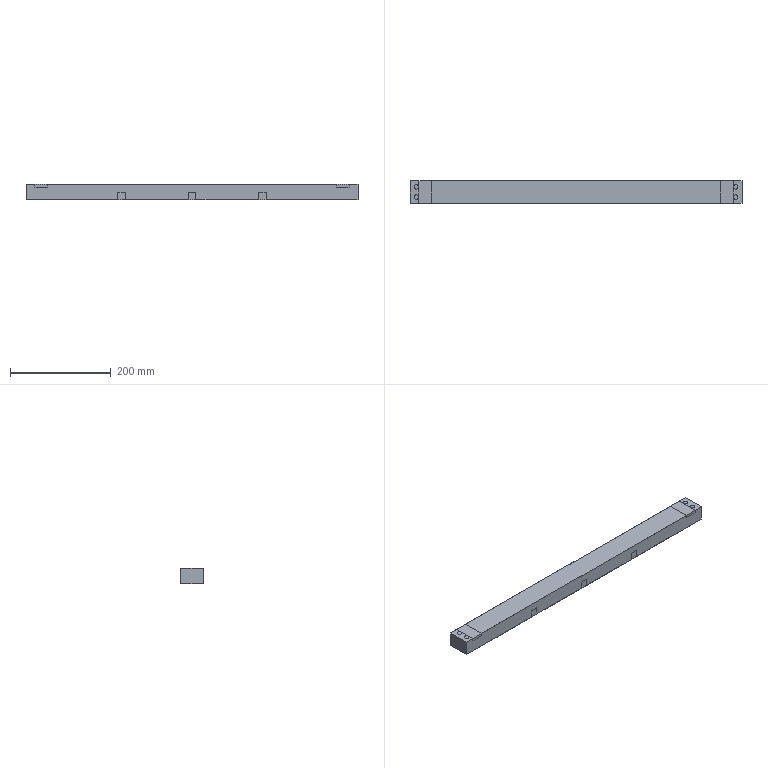NC program | NX | posted with a generic post | part box 659.9 x 45 x 30 mm
Whole program:
N10 G17 G21 G94 G90
(FLOOR_WALL , TOOL : D63)
N12 T01 M6
N14 G54
N16 G17 G0 G90 X-366.45 Y0. S6500 M3
N18 G43 Z30. H1
N20 Z3.
N22 G94 G1 Z0. F1250.
N24 X-363.45
N26 X363.45
N28 X366.45
N30 Z3.
N32 G0 Z30.
N34 M5
(ZLEVEL_PROFILE_COPY_2 , TOOL : D12)
N36 T20 M6
N38 G54
N40 G17 G0 G90 X338.221 Y33.444 S8000 M3
N42 G43 Z30. H20
N44 Z-1.
N46 G94 G1 X336.646 Y32.535 F3500.
N48 G3 X336.046 Y31.496 R1.2
N50 G1 Y23.409
N52 X336.05 Y22.53
N54 Y-17.291
N56 X336.046 Y-17.344
N58 Y-31.496
N60 G3 X336.646 Y-32.535 R1.2
N62 G1 X338.221 Y-33.444
N64 G0 Z-2.
N66 G1 X336.646 Y-32.535
N68 G2 X336.046 Y-31.496 R1.2
N70 G1 Y-17.344
N72 X336.05 Y-17.291
N74 Y22.53
N76 X336.046 Y23.409
N78 Y31.496
N80 G2 X336.646 Y32.535 R1.2
N82 G1 X338.221 Y33.444
N84 G0 Z-3.
N86 G1 X336.646 Y32.535
N88 G3 X336.046 Y31.496 R1.2
N90 G1 Y23.409
N92 X336.05 Y22.53
N94 Y-17.291
N96 X336.046 Y-17.344
N98 Y-31.496
N100 G3 X336.646 Y-32.535 R1.2
N102 G1 X338.221 Y-33.444
N104 G0 Z-4.
N106 G1 X336.646 Y-32.535
N108 G2 X336.046 Y-31.496 R1.2
N110 G1 Y-17.344
N112 X336.05 Y-17.291
N114 Y22.53
N116 X336.046 Y23.409
N118 Y31.496
N120 G2 X336.646 Y32.535 R1.2
N122 G1 X338.221 Y33.444
N124 G0 Z-5.
N126 G1 X336.646 Y32.535
N128 G3 X336.046 Y31.496 R1.2
N130 G1 Y23.409
N132 X336.05 Y22.53
N134 Y-17.291
N136 X336.046 Y-17.344
N138 Y-31.496
N140 G3 X336.646 Y-32.535 R1.2
N142 G1 X338.221 Y-33.444
N144 G0 Z-6.
N146 G1 X336.646 Y-32.535
N148 G2 X336.046 Y-31.496 R1.2
N150 G1 Y-17.344
N152 X336.05 Y-17.291
N154 Y22.53
N156 X336.046 Y23.409
N158 Y31.496
N160 G2 X336.646 Y32.535 R1.2
N162 G1 X338.221 Y33.444
N164 G0 Z-7.
N166 G1 X336.646 Y32.535
N168 G3 X336.046 Y31.496 R1.2
N170 G1 Y23.409
N172 X336.05 Y22.53
N174 Y-17.291
N176 X336.046 Y-17.344
N178 Y-31.496
N180 G3 X336.646 Y-32.535 R1.2
N182 G1 X338.221 Y-33.444
N184 G0 Z-8.
N186 G1 X336.647 Y-32.535
N188 G2 X336.047 Y-31.496 R1.2
N190 G1 Y-17.344
N192 X336.05 Y-17.291
N194 Y22.53
N196 X336.047 Y23.409
N198 Y31.496
N200 G2 X336.647 Y32.535 R1.2
N202 G1 X338.221 Y33.444
N204 G0 Z-9.
N206 G1 X336.647 Y32.535
N208 G3 X336.047 Y31.496 R1.2
N210 G1 Y23.409
N212 X336.05 Y22.53
N214 Y-17.291
N216 X336.047 Y-17.344
N218 Y-31.496
N220 G3 X336.647 Y-32.535 R1.2
N222 G1 X338.221 Y-33.444
N224 G0 Z-10.
N226 G1 X336.647 Y-32.535
N228 G2 X336.047 Y-31.496 R1.2
N230 G1 Y-17.344
N232 X336.05 Y-17.291
N234 Y22.53
N236 X336.047 Y23.409
N238 Y31.496
N240 G2 X336.647 Y32.535 R1.2
N242 G1 X338.221 Y33.444
N244 G0 Z-11.
N246 G1 X336.647 Y32.535
N248 G3 X336.047 Y31.496 R1.2
N250 G1 Y23.409
N252 X336.05 Y22.53
N254 Y-17.291
N256 X336.047 Y-17.344
N258 Y-31.496
N260 G3 X336.647 Y-32.535 R1.2
N262 G1 X338.221 Y-33.444
N264 G0 Z-12.
N266 G1 X336.647 Y-32.535
N268 G2 X336.047 Y-31.496 R1.2
N270 G1 Y-17.344
N272 X336.05 Y-17.291
N274 Y22.53
N276 X336.047 Y23.409
N278 Y31.496
N280 G2 X336.647 Y32.535 R1.2
N282 G1 X338.222 Y33.444
N284 G0 Z-13.
N286 G1 X336.647 Y32.535
N288 G3 X336.047 Y31.496 R1.2
N290 G1 Y23.409
N292 X336.05 Y22.53
N294 X336.047 Y-17.344
N296 Y-31.496
N298 G3 X336.647 Y-32.535 R1.2
N300 G1 X338.222 Y-33.444
N302 G0 Z-14.
N304 G1 X336.647 Y-32.535
N306 G2 X336.047 Y-31.496 R1.2
N308 G1 X336.05 Y-17.291
N310 Y22.53
N312 X336.047 Y23.409
N314 Y31.496
N316 G2 X336.647 Y32.535 R1.2
N318 G1 X338.222 Y33.444
N320 G0 Z-15.
N322 G1 X336.647 Y32.535
N324 G3 X336.047 Y31.496 R1.2
N326 G1 Y23.409
N328 X336.05 Y22.53
N330 X336.047 Y-17.344
N332 Y-31.496
N334 G3 X336.647 Y-32.535 R1.2
N336 G1 X338.222 Y-33.444
N338 G0 Z-16.
N340 G1 X336.647 Y-32.535
N342 G2 X336.047 Y-31.496 R1.2
N344 G1 X336.05 Y-17.291
N346 Y22.53
N348 X336.047 Y23.409
N350 Y31.496
N352 G2 X336.647 Y32.535 R1.2
N354 G1 X338.222 Y33.444
N356 G0 Z-17.
N358 G1 X336.647 Y32.535
N360 G3 X336.047 Y31.496 R1.2
N362 G1 Y23.409
N364 X336.05 Y22.53
N366 X336.047 Y-17.344
N368 Y-31.496
N370 G3 X336.647 Y-32.535 R1.2
N372 G1 X338.222 Y-33.444
N374 G0 Z-18.
N376 G1 X336.647 Y-32.535
N378 G2 X336.047 Y-31.496 R1.2
N380 G1 X336.05 Y-17.291
N382 Y22.53
N384 X336.047 Y23.409
N386 Y31.496
N388 G2 X336.647 Y32.535 R1.2
N390 G1 X338.222 Y33.444
N392 G0 Z-19.
N394 G1 X336.648 Y32.535
N396 G3 X336.048 Y31.496 R1.2
N398 G1 Y23.409
N400 X336.05 Y22.53
N402 X336.048 Y-17.344
N404 Y-31.496
N406 G3 X336.648 Y-32.535 R1.2
N408 G1 X338.222 Y-33.444
N410 G0 Z-20.
N412 G1 X336.648 Y-32.535
N414 G2 X336.048 Y-31.496 R1.2
N416 G1 X336.05 Y-17.291
N418 Y22.53
N420 X336.048 Y23.409
N422 Y31.496
N424 G2 X336.648 Y32.535 R1.2
N426 G1 X338.222 Y33.444
N428 G0 Z-21.
N430 G1 X336.648 Y32.535
N432 G3 X336.048 Y31.496 R1.2
N434 G1 Y23.409
N436 X336.05 Y22.53
N438 X336.048 Y-17.344
N440 Y-31.496
N442 G3 X336.648 Y-32.535 R1.2
N444 G1 X338.222 Y-33.444
N446 G0 Z-22.
N448 G1 X336.648 Y-32.535
N450 G2 X336.048 Y-31.496 R1.2
N452 G1 X336.05 Y-17.291
N454 Y22.53
N456 X336.048 Y23.409
N458 Y31.496
N460 G2 X336.648 Y32.535 R1.2
N462 G1 X338.222 Y33.444
N464 G0 Y33.445 Z-23.
N466 G1 X336.648 Y32.536
N468 G3 X336.048 Y31.496 R1.2
N470 G1 X336.05 Y22.53
N472 X336.048 Y-17.344
N474 Y-31.496
N476 G3 X336.648 Y-32.535 R1.2
N478 G1 X338.222 Y-33.444
N480 G0 Z-24.
N482 G1 X336.648 Y-32.535
N484 G2 X336.048 Y-31.496 R1.2
N486 G1 X336.05 Y-17.291
N488 Y22.53
N490 X336.048 Y31.496
N492 G2 X336.648 Y32.536 R1.2
N494 G1 X338.222 Y33.445
N496 G0 Z-25.
N498 G1 X336.648 Y32.536
N500 G3 X336.048 Y31.496 R1.2
N502 G1 X336.05 Y22.53
N504 X336.048 Y-17.344
N506 Y-31.496
N508 G3 X336.648 Y-32.535 R1.2
N510 G1 X338.222 Y-33.444
N512 G0 X338.223 Y-33.445 Z-26.
N514 G1 X336.648 Y-32.535
N516 G2 X336.048 Y-31.496 R1.2
N518 G1 X336.05 Y-17.291
N520 Y22.53
N522 X336.048 Y31.496
N524 G2 X336.648 Y32.536 R1.2
N526 G1 X338.223 Y33.445
N528 G0 Z-27.
N530 G1 X336.648 Y32.536
N532 G3 X336.048 Y31.496 R1.2
N534 G1 X336.05 Y22.53
N536 Y-17.291
N538 X336.048 Y-31.496
N540 G3 X336.648 Y-32.535 R1.2
N542 G1 X338.223 Y-33.445
N544 G0 Z-28.
N546 G1 X336.648 Y-32.535
N548 G2 X336.048 Y-31.496 R1.2
N550 G1 X336.05 Y-17.291
N552 Y22.53
N554 X336.048 Y31.496
N556 G2 X336.648 Y32.536 R1.2
N558 G1 X338.223 Y33.445
N560 G0 Z-29.
N562 G1 X336.648 Y32.536
N564 G3 X336.048 Y31.496 R1.2
N566 G1 X336.05 Y22.53
N568 Y-17.291
N570 X336.048 Y-31.496
N572 G3 X336.648 Y-32.536 R1.2
N574 G1 X338.223 Y-33.445
N576 G0 Z-30.
N578 G1 X336.648 Y-32.536
N580 G2 X336.049 Y-31.496 R1.2
N582 G1 X336.05 Y-17.291
N584 Y22.53
N586 X336.049 Y31.496
N588 G2 X336.648 Y32.536 R1.2
N590 G1 X338.223 Y33.445
N592 G0 Z30.
N594 X-338.221 Y-33.444
N596 Z-1.
N598 G1 X-336.646 Y-32.535
N600 G3 X-336.046 Y-31.496 R1.2
N602 G1 Y-17.344
N604 X-336.05 Y-17.291
N606 Y22.5
N608 X-336.022 Y23.088
N610 X-336.046 Y23.143
N612 Y31.496
N614 G3 X-336.646 Y32.535 R1.2
N616 G1 X-338.221 Y33.444
N618 G0 Z-2.
N620 G1 X-336.646 Y32.535
N622 G2 X-336.046 Y31.496 R1.2
N624 G1 Y23.143
N626 X-336.022 Y23.088
N628 X-336.05 Y22.5
N630 Y-17.291
N632 X-336.046 Y-17.344
N634 Y-31.496
N636 G2 X-336.646 Y-32.535 R1.2
N638 G1 X-338.221 Y-33.444
N640 G0 Z-3.
N642 G1 X-336.646 Y-32.535
N644 G3 X-336.046 Y-31.496 R1.2
N646 G1 Y-17.344
N648 X-336.05 Y-17.291
N650 Y22.5
N652 X-336.022 Y23.088
N654 X-336.046 Y23.143
N656 Y31.496
N658 G3 X-336.646 Y32.535 R1.2
N660 G1 X-338.221 Y33.444
N662 G0 Z-4.
N664 G1 X-336.646 Y32.535
N666 G2 X-336.046 Y31.496 R1.2
N668 G1 Y23.143
N670 X-336.022 Y23.088
N672 X-336.05 Y22.5
N674 Y-17.291
N676 X-336.046 Y-17.344
N678 Y-31.496
N680 G2 X-336.646 Y-32.535 R1.2
N682 G1 X-338.221 Y-33.444
N684 G0 Z-5.
N686 G1 X-336.646 Y-32.535
N688 G3 X-336.046 Y-31.496 R1.2
N690 G1 Y-17.344
N692 X-336.05 Y-17.291
N694 Y22.5
N696 X-336.022 Y23.088
N698 X-336.046 Y23.143
N700 Y31.496
N702 G3 X-336.646 Y32.535 R1.2
N704 G1 X-338.221 Y33.444
N706 G0 Z-6.
N708 G1 X-336.646 Y32.535
N710 G2 X-336.046 Y31.496 R1.2
N712 G1 Y23.143
N714 X-336.022 Y23.088
N716 X-336.05 Y22.5
N718 Y-17.291
N720 X-336.046 Y-17.344
N722 Y-31.496
N724 G2 X-336.646 Y-32.535 R1.2
N726 G1 X-338.221 Y-33.444
N728 G0 Z-7.
N730 G1 X-336.646 Y-32.535
N732 G3 X-336.046 Y-31.496 R1.2
N734 G1 Y-17.344
N736 X-336.05 Y-17.291
N738 Y22.5
N740 X-336.022 Y23.088
N742 X-336.046 Y23.143
N744 Y31.496
N746 G3 X-336.646 Y32.535 R1.2
N748 G1 X-338.221 Y33.444
N750 G0 Z-8.
N752 G1 X-336.647 Y32.535
N754 G2 X-336.047 Y31.496 R1.2
N756 G1 Y23.143
N758 X-336.022 Y23.088
N760 X-336.05 Y22.5
N762 Y-17.291
N764 X-336.047 Y-17.344
N766 Y-31.496
N768 G2 X-336.647 Y-32.535 R1.2
N770 G1 X-338.221 Y-33.444
N772 G0 Z-9.
N774 G1 X-336.647 Y-32.535
N776 G3 X-336.047 Y-31.496 R1.2
N778 G1 Y-17.344
N780 X-336.05 Y-17.291
N782 Y22.5
N784 X-336.022 Y23.088
N786 X-336.047 Y23.143
N788 Y31.496
N790 G3 X-336.647 Y32.535 R1.2
N792 G1 X-338.221 Y33.444
N794 G0 Z-10.
N796 G1 X-336.647 Y32.535
N798 G2 X-336.047 Y31.496 R1.2
N800 G1 Y23.143
N802 X-336.022 Y23.088
N804 X-336.05 Y22.5
N806 Y-17.291
N808 X-336.047 Y-17.344
N810 Y-31.496
N812 G2 X-336.647 Y-32.535 R1.2
N814 G1 X-338.221 Y-33.444
N816 G0 Z-11.
N818 G1 X-336.647 Y-32.535
N820 G3 X-336.047 Y-31.496 R1.2
N822 G1 Y-17.344
N824 X-336.05 Y-17.291
N826 Y22.5
N828 X-336.022 Y23.088
N830 X-336.047 Y23.143
N832 Y31.496
N834 G3 X-336.647 Y32.535 R1.2
N836 G1 X-338.221 Y33.444
N838 G0 Z-12.
N840 G1 X-336.647 Y32.535
N842 G2 X-336.047 Y31.496 R1.2
N844 G1 Y23.143
N846 X-336.022 Y23.088
N848 X-336.05 Y22.5
N850 Y-17.291
N852 X-336.047 Y-17.344
N854 Y-31.496
N856 G2 X-336.647 Y-32.535 R1.2
N858 G1 X-338.222 Y-33.444
N860 G0 Z-13.
N862 G1 X-336.647 Y-32.535
N864 G3 X-336.047 Y-31.496 R1.2
N866 G1 X-336.05 Y-17.291
N868 Y22.5
N870 X-336.022 Y23.088
N872 X-336.047 Y23.143
N874 Y31.496
N876 G3 X-336.647 Y32.535 R1.2
N878 G1 X-338.222 Y33.444
N880 G0 Z-14.
N882 G1 X-336.647 Y32.535
N884 G2 X-336.047 Y31.496 R1.2
N886 G1 Y23.143
N888 X-336.022 Y23.088
N890 X-336.05 Y22.5
N892 X-336.047 Y-17.344
N894 Y-31.496
N896 G2 X-336.647 Y-32.535 R1.2
N898 G1 X-338.222 Y-33.444
N900 G0 Z-15.
N902 G1 X-336.647 Y-32.535
N904 G3 X-336.047 Y-31.496 R1.2
N906 G1 X-336.05 Y-17.291
N908 Y22.5
N910 X-336.022 Y23.088
N912 X-336.047 Y23.143
N914 Y31.496
N916 G3 X-336.647 Y32.535 R1.2
N918 G1 X-338.222 Y33.444
N920 G0 Z-16.
N922 G1 X-336.647 Y32.535
N924 G2 X-336.047 Y31.496 R1.2
N926 G1 Y23.143
N928 X-336.022 Y23.088
N930 X-336.05 Y22.5
N932 X-336.047 Y-17.344
N934 Y-31.496
N936 G2 X-336.647 Y-32.535 R1.2
N938 G1 X-338.222 Y-33.444
N940 G0 Z-17.
N942 G1 X-336.647 Y-32.535
N944 G3 X-336.047 Y-31.496 R1.2
N946 G1 X-336.05 Y-17.291
N948 Y22.5
N950 X-336.022 Y23.088
N952 X-336.047 Y23.143
N954 Y31.496
N956 G3 X-336.647 Y32.535 R1.2
N958 G1 X-338.222 Y33.444
N960 G0 Z-18.
N962 G1 X-336.647 Y32.535
N964 G2 X-336.047 Y31.496 R1.2
N966 G1 Y23.143
N968 X-336.022 Y23.088
N970 X-336.05 Y22.5
N972 X-336.047 Y-17.344
N974 Y-31.496
N976 G2 X-336.647 Y-32.535 R1.2
N978 G1 X-338.222 Y-33.444
N980 G0 Z-19.
N982 G1 X-336.648 Y-32.535
N984 G3 X-336.048 Y-31.496 R1.2
N986 G1 X-336.05 Y-17.291
N988 Y22.5
N990 X-336.022 Y23.088
N992 X-336.048 Y23.143
N994 Y31.496
N996 G3 X-336.648 Y32.535 R1.2
N998 G1 X-338.222 Y33.444
N1000 G0 Z-20.
N1002 G1 X-336.648 Y32.535
N1004 G2 X-336.048 Y31.496 R1.2
N1006 G1 Y23.143
N1008 X-336.022 Y23.088
N1010 X-336.05 Y22.5
N1012 X-336.048 Y-17.344
N1014 Y-31.496
N1016 G2 X-336.648 Y-32.535 R1.2
N1018 G1 X-338.222 Y-33.444
N1020 G0 Z-21.
N1022 G1 X-336.648 Y-32.535
N1024 G3 X-336.048 Y-31.496 R1.2
N1026 G1 X-336.05 Y-17.291
N1028 Y22.5
N1030 X-336.022 Y23.088
N1032 X-336.048 Y23.143
N1034 Y31.496
N1036 G3 X-336.648 Y32.535 R1.2
N1038 G1 X-338.222 Y33.444
N1040 G0 Z-22.
N1042 G1 X-336.648 Y32.535
N1044 G2 X-336.048 Y31.496 R1.2
N1046 G1 Y23.143
N1048 X-336.022 Y23.088
N1050 X-336.05 Y22.5
N1052 X-336.048 Y-17.344
N1054 Y-31.496
N1056 G2 X-336.648 Y-32.535 R1.2
N1058 G1 X-338.222 Y-33.444
N1060 G0 Z-23.
N1062 G1 X-336.648 Y-32.535
N1064 G3 X-336.048 Y-31.496 R1.2
N1066 G1 X-336.05 Y-17.291
N1068 Y22.5
N1070 X-336.022 Y23.088
N1072 X-336.048 Y23.143
N1074 Y31.496
N1076 G3 X-336.648 Y32.535 R1.2
N1078 G1 X-338.222 Y33.444
N1080 G0 Z-24.
N1082 G1 X-336.648 Y32.535
N1084 G2 X-336.048 Y31.496 R1.2
N1086 G1 Y23.143
N1088 X-336.022 Y23.088
N1090 X-336.05 Y22.5
N1092 X-336.048 Y-17.344
N1094 Y-31.496
N1096 G2 X-336.648 Y-32.535 R1.2
N1098 G1 X-338.222 Y-33.444
N1100 G0 X-338.223 Z-25.
N1102 G1 X-336.648 Y-32.535
N1104 G3 X-336.048 Y-31.496 R1.2
N1106 G1 X-336.05 Y-17.291
N1108 Y22.5
N1110 X-336.022 Y23.088
N1112 X-336.048 Y23.143
N1114 Y31.496
N1116 G3 X-336.648 Y32.535 R1.2
N1118 G1 X-338.222 Y33.444
N1120 G0 X-338.223 Z-26.
N1122 G1 X-336.648 Y32.535
N1124 G2 X-336.048 Y31.496 R1.2
N1126 G1 Y23.143
N1128 X-336.022 Y23.088
N1130 X-336.05 Y22.5
N1132 Y-17.291
N1134 X-336.048 Y-31.496
N1136 G2 X-336.648 Y-32.535 R1.2
N1138 G1 X-338.223 Y-33.445
N1140 G0 Z-27.
N1142 G1 X-336.648 Y-32.535
N1144 G3 X-336.048 Y-31.496 R1.2
N1146 G1 X-336.05 Y-17.291
N1148 Y22.5
N1150 X-336.022 Y23.088
N1152 X-336.048 Y23.143
N1154 Y31.496
N1156 G3 X-336.648 Y32.535 R1.2
N1158 G1 X-338.223 Y33.444
N1160 G0 Z-28.
N1162 G1 X-336.648 Y32.535
N1164 G2 X-336.048 Y31.496 R1.2
N1166 G1 Y23.143
N1168 X-336.022 Y23.088
N1170 X-336.05 Y22.5
N1172 Y-17.291
N1174 X-336.048 Y-31.496
N1176 G2 X-336.648 Y-32.535 R1.2
N1178 G1 X-338.223 Y-33.445
N1180 G0 Z-29.
N1182 G1 X-336.648 Y-32.536
N1184 G3 X-336.048 Y-31.496 R1.2
N1186 G1 X-336.05 Y-17.291
N1188 Y22.5
N1190 X-336.022 Y23.088
N1192 X-336.048 Y23.143
N1194 Y31.496
N1196 G3 X-336.648 Y32.535 R1.2
N1198 G1 X-338.223 Y33.444
N1200 G0 Z-30.
N1202 G1 X-336.649 Y32.535
N1204 G2 X-336.049 Y31.496 R1.2
N1206 G1 Y23.143
N1208 X-336.022 Y23.088
N1210 X-336.05 Y22.5
N1212 Y-17.291
N1214 X-336.049 Y-31.496
N1216 G2 X-336.648 Y-32.536 R1.2
N1218 G1 X-338.223 Y-33.445
N1220 G0 Z30.
(FLOOR_WALL_1_2 , TOOL : D12)
N1222 X-299.5 Y30.
N1224 Z0.25
N1226 G1 Z-1.25 F1000.
N1228 Y22.5
N1230 X-293. F3000.
N1232 Y-22.5
N1234 X-306.
N1236 Y22.5
N1238 X-299.5
N1240 Y17.1
N1242 X-298.4
N1244 Y-17.1
N1246 X-300.6
N1248 Y17.1
N1250 X-299.5
N1252 Y20.1
N1254 Y30.
N1256 Z0.25
N1258 G0 Z-1.
N1260 G1 Z-2.5 F1000.
N1262 Y22.5
N1264 X-293. F3000.
N1266 Y-22.5
N1268 X-306.
N1270 Y22.5
N1272 X-299.5
N1274 Y17.1
N1276 X-298.4
N1278 Y-17.1
N1280 X-300.6
N1282 Y17.1
N1284 X-299.5
N1286 Y20.1
N1288 Y30.
N1290 Z-1.
N1292 G0 Z-2.25
N1294 G1 Z-3.75 F1000.
N1296 Y22.5
N1298 X-293. F3000.
N1300 Y-22.5
N1302 X-306.
N1304 Y22.5
N1306 X-299.5
N1308 Y17.1
N1310 X-298.4
N1312 Y-17.1
N1314 X-300.6
N1316 Y17.1
N1318 X-299.5
N1320 Y20.1
N1322 Y30.
N1324 Z-2.25
N1326 G0 Z-3.5
N1328 G1 Z-5. F1000.
N1330 Y22.5
N1332 X-293. F3000.
N1334 Y-22.5
N1336 X-306.
N1338 Y22.5
N1340 X-299.5
N1342 Y17.1
N1344 X-298.4
N1346 Y-17.1
N1348 X-300.6
N1350 Y17.1
N1352 X-299.5
N1354 Y20.1
N1356 Y30.
N1358 Z-3.5
N1360 G0 Z30.
N1362 X299.5 Y-30.
N1364 Z0.25
N1366 G1 Z-1.25 F1000.
N1368 Y-22.5
N1370 X293. F3000.
N1372 Y22.5
N1374 X306.
N1376 Y-22.5
N1378 X299.5
N1380 Y-17.1
N1382 X298.4
N1384 Y17.1
N1386 X300.6
N1388 Y-17.1
N1390 X299.5
N1392 Y-30.
N1394 Z0.25
N1396 G0 Z-1.
N1398 G1 Z-2.5 F1000.
N1400 Y-22.5
N1402 X293. F3000.
N1404 Y22.5
N1406 X306.
N1408 Y-22.5
N1410 X299.5
N1412 Y-17.1
N1414 X298.4
N1416 Y17.1
N1418 X300.6
N1420 Y-17.1
N1422 X299.5
N1424 Y-30.
N1426 Z-1.
N1428 G0 Z-2.25
N1430 G1 Z-3.75 F1000.
N1432 Y-22.5
N1434 X293. F3000.
N1436 Y22.5
N1438 X306.
N1440 Y-22.5
N1442 X299.5
N1444 Y-17.1
N1446 X298.4
N1448 Y17.1
N1450 X300.6
N1452 Y-17.1
N1454 X299.5
N1456 Y-30.
N1458 Z-2.25
N1460 G0 Z-3.5
N1462 G1 Z-5. F1000.
N1464 Y-22.5
N1466 X293. F3000.
N1468 Y22.5
N1470 X306.
N1472 Y-22.5
N1474 X299.5
N1476 Y-17.1
N1478 X298.4
N1480 Y17.1
N1482 X300.6
N1484 Y-17.1
N1486 X299.5
N1488 Y-30.
N1490 Z-3.5
N1492 G0 Z30.
N1494 M5
(DRILLING_COPY_1 , TOOL : D6A45)
N1496 T02 M6
N1498 G54
N1500 G17 G0 G90 X-317.5 Y10. S3000 M3
N1502 G43 Z30. H2
N1504 G94 G81 G98 Z-1. F200. R3.
N1506 Y-10.
N1508 X-306.5 Y0. Z-6.1 R-2.1
N1510 X-295.5 Y-10.
N1512 Y10.
N1514 X295.5
N1516 Y-10.
N1518 X306.5 Y0.
N1520 X317.5 Y-10. Z-1. R3.
N1522 Y10.
N1524 G80
N1526 G0 X317.5 Y10. Z30.
N1528 M5
(DRILLING_COPY_COPY_1 , TOOL : 9.0ZT)
N1530 T09 M6
N1532 G54
N1534 G17 G0 G90 X-317.5 Y10. S1500 M3
N1536 G43 Z30. H9
N1538 G94 G83 G98 Z-30. F200. Q2. R3.
N1540 Y-10.
N1542 X-295.5 R-2.1
N1544 Y10.
N1546 X295.5 Y-10.
N1548 Y10.
N1550 X317.5 R3.
N1552 Y-10.
N1554 G80
N1556 G0 X317.5 Y-10. Z30.
N1558 M5
(DRILLING_COPY_COPY_COPY_1 , TOOL : 7.8ZT)
N1560 T12 M6
N1562 G54
N1564 G17 G0 G90 X-306.5 Y0. S1500 M3
N1566 G43 Z30. H12
N1568 G94 G83 G98 Z-33.843 F200. Q2. R-2.1
N1570 X306.5
N1572 G80
N1574 G0 X306.5 Y0. Z30.
N1576 M5
(DRILLING_COPY_COPY_COPY_COPY_1 , TOOL : 8.0JD)
N1578 T13 M6
N1580 G54
N1582 G17 G0 G90 X-306.5 Y0. S1000 M3
N1584 G43 Z30. H13
N1586 G94 G85 G98 Z-30.5 F50. R-2.1
N1588 X306.5
N1590 G80
N1592 G0 X306.5 Y0. Z30.
N1594 M5
(FLOOR_WALL_1_COPY , TOOL : D12JING)
N1596 T21 M6
N1598 G54
N1600 G17 G0 G90 X-306.099 Y-30. S8000 M3
N1602 G43 Z30. H21
N1604 Z-3.6
N1606 G94 G1 Z-5.1 F1000.
N1608 Y-28.5
N1610 Y28.5 F1200.
N1612 X-299.5
N1614 Y-28.5
N1616 X-292.9
N1618 Y28.5
N1620 Y30.
N1622 Z-3.6
N1624 G0 Z30.
N1626 X292.901 Y-30.
N1628 Z-3.6
N1630 G1 Z-5.1 F1000.
N1632 Y-28.5
N1634 Y28.5 F1200.
N1636 X299.5
N1638 Y-28.5
N1640 X306.1
N1642 Y28.5
N1644 Y30.
N1646 Z-3.6
N1648 G0 Z30.
(CUTTERCOMP11_COPY , TOOL : D12JING)
N1650 X338.27 Y30.826
N1652 Z-14.
N1654 G1 Z-15.
N1656 G41 X338.176 Y30.791 D21
N1658 X336.549 Y29.852
N1660 G3 X335.949 Y28.813 R1.2
N1662 G1 X335.948 Y23.013
N1664 X335.95 Y22.514
N1666 Y-20.618
N1668 X335.949 Y-20.633
N1670 Y-28.813
N1672 G3 X336.549 Y-29.852 R1.2
N1674 G1 X338.178 Y-30.792
N1676 G40
N1678 X338.272 Y-30.827
N1680 Z-14.
N1682 G0 X338.271 Y30.826 Z-29.
N1684 G1 Z-30.
N1686 G41 X338.177 Y30.792
N1688 X336.55 Y29.852
N1690 G3 X335.95 Y28.813 R1.2
N1692 G1 Y22.514
N1694 Y-20.618
N1696 Y-28.813
N1698 G3 X336.55 Y-29.852 R1.2
N1700 G1 X338.179 Y-30.793
N1702 G40
N1704 X338.273 Y-30.827
N1706 Z-29.
N1708 G0 Z30.
N1710 X-338.271
N1712 Z-14.
N1714 G1 Z-15.
N1716 G41 X-338.177 Y-30.793
N1718 X-336.548 Y-29.852
N1720 G3 X-335.948 Y-28.813 R1.2
N1722 G1 X-335.949 Y-20.633
N1724 X-335.95 Y-20.618
N1726 Y22.5
N1728 X-335.948 Y22.861
N1730 Y28.813
N1732 G3 X-336.548 Y29.852 R1.2
N1734 G1 X-338.177 Y30.792
N1736 G40
N1738 X-338.271 Y30.826
N1740 Z-14.
N1742 G0 X-338.272 Y-30.827 Z-29.
N1744 G1 Z-30.
N1746 G41 X-338.178 Y-30.792
N1748 X-336.549 Y-29.852
N1750 G3 X-335.949 Y-28.813 R1.2
N1752 G1 Y-20.999
N1754 X-335.95 Y-20.618
N1756 Y22.5
N1758 X-335.949 Y22.952
N1760 Y28.813
N1762 G3 X-336.549 Y29.852 R1.2
N1764 G1 X-338.177 Y30.792
N1766 G40
N1768 X-338.271 Y30.826
N1770 Z-29.
N1772 G0 Z30.
(CUTTERCOMP11_COPY_COPY , TOOL : D12JING)
N1774 X303.84 Y-31.102
N1776 Z-4.1
N1778 G1 Z-5.1
N1780 G41 X303.934 Y-31.067
N1782 X305.509 Y-30.142
N1784 G3 X306.101 Y-29.098 R1.2
N1786 G1 X306.098 Y-28.813
N1788 Y-22.952
N1790 X306.1 Y-21.976
N1792 Y22.482
N1794 X306.098 Y22.5
N1796 X306.118 Y22.966
N1798 X306.098 Y22.983
N1800 Y28.813
N1802 X306.101 Y29.098
N1804 G3 X305.509 Y30.142 R1.2
N1806 G1 X303.934 Y31.067
N1808 G40
N1810 X303.84 Y31.102
N1812 Z-4.1
N1814 G0 Z30.
N1816 X295.166 Y31.079
N1818 Z-4.1
N1820 G1 Z-5.1
N1822 G41 X295.072 Y31.045
N1824 X293.499 Y30.137
N1826 G3 X292.899 Y29.098 R1.2
N1828 G1 X292.9 Y22.482
N1830 Y-21.976
N1832 X292.902 Y-22.952
N1834 Y-28.813
N1836 X292.899 Y-29.098
N1838 G3 X293.491 Y-30.142 R1.2
N1840 G1 X295.066 Y-31.067
N1842 G40
N1844 X295.16 Y-31.102
N1846 Z-4.1
N1848 G0 Z30.
N1850 X-295.16
N1852 Z-4.1
N1854 G1 Z-5.1
N1856 G41 X-295.066 Y-31.067
N1858 X-293.491 Y-30.142
N1860 G3 X-292.899 Y-29.098 R1.2
N1862 G1 X-292.902 Y-28.813
N1864 Y-22.952
N1866 X-292.9 Y-21.976
N1868 Y22.482
N1870 X-292.902 Y22.5
N1872 X-292.882 Y22.966
N1874 X-292.902 Y22.983
N1876 Y28.813
N1878 X-292.899 Y29.098
N1880 G3 X-293.491 Y30.142 R1.2
N1882 G1 X-295.066 Y31.067
N1884 G40
N1886 X-295.16 Y31.102
N1888 Z-4.1
N1890 G0 Z30.
N1892 X-303.834 Y31.079
N1894 Z-4.1
N1896 G1 Z-5.1
N1898 G41 X-303.928 Y31.045
N1900 X-305.501 Y30.137
N1902 G3 X-306.101 Y29.098 R1.2
N1904 G1 X-306.1 Y22.482
N1906 Y-21.976
N1908 X-306.098 Y-22.952
N1910 Y-28.813
N1912 X-306.101 Y-29.098
N1914 G3 X-305.509 Y-30.142 R1.2
N1916 G1 X-303.934 Y-31.067
N1918 G40
N1920 X-303.84 Y-31.102
N1922 Z-4.1
N1924 G0 Z30.
N1926 M5
(ZLEVEL_PROFILE_COPY_1_COPY_COPY_COPY_COPY_2 , TOOL : D6A45)
N1928 T02 M6
N1930 G54
N1932 G17 G0 G90 X-319.688 Y11.223 S7000 M3
N1934 G43 Z30. H2
N1936 Z-1.
N1938 G94 G1 X-320.907 Y10.52 F1000.
N1940 G3 X-321.207 Y10. R0.6
N1942 X-317.5 Y6.293 R3.707
N1944 X-321.207 Y10. R-3.707
N1946 X-320.907 Y9.48 R0.6
N1948 G1 X-319.688 Y8.777
N1950 G0 Z30.
N1952 Y-8.777
N1954 Z-1.
N1956 G1 X-320.907 Y-9.48
N1958 G3 X-321.207 Y-10. R0.6
N1960 X-317.5 Y-13.707 R3.707
N1962 X-321.207 Y-10. R-3.707
N1964 X-320.907 Y-10.52 R0.6
N1966 G1 X-319.688 Y-11.223
N1968 G0 Z30.
N1970 X316.277 Y-12.188
N1972 Z-1.
N1974 G1 X316.98 Y-13.407
N1976 G3 X317.5 Y-13.707 R0.6
N1978 X321.207 Y-10. R3.707
N1980 X317.5 Y-13.707 R-3.707
N1982 X318.02 Y-13.407 R0.6
N1984 G1 X318.723 Y-12.188
N1986 G0 Z30.
N1988 X319.688 Y8.777
N1990 Z-1.
N1992 G1 X320.907 Y9.48
N1994 G3 X321.207 Y10. R0.6
N1996 X317.5 Y13.707 R3.707
N1998 X321.207 Y10. R-3.707
N2000 X320.907 Y10.52 R0.6
N2002 G1 X319.688 Y11.223
N2004 G0 Z30.
N2006 X-287.813 Y24.272
N2008 Z-1.
N2010 G1 X-287.421 Y23.593
N2012 G3 X-286.901 Y23.293 R0.6
N2014 G1 X286.901
N2016 G2 X287.693 Y22.501 R0.792
N2018 G1 Y-22.501
N2020 G2 X286.901 Y-23.293 R0.792
N2022 G1 X-286.901
N2024 G2 X-287.693 Y-22.501 R0.792
N2026 G1 Y22.501
N2028 G2 X-286.901 Y23.293 R0.792
N2030 G3 X-286.381 Y23.593 R0.6
N2032 G1 X-285.862 Y24.493
N2034 G0 Z30.
N2036 X331.722 Y23.413
N2038 Z-1.
N2040 G1 X331.043 Y23.02
N2042 G3 X330.743 Y22.501 R0.6
N2044 G1 Y-22.501
N2046 G2 X329.951 Y-23.293 R0.792
N2048 G1 X312.099
N2050 G2 X311.307 Y-22.501 R0.792
N2052 G1 Y22.501
N2054 G2 X312.099 Y23.293 R0.792
N2056 G1 X329.951
N2058 G2 X330.743 Y22.501 R0.792
N2060 G3 X331.043 Y21.981 R0.6
N2062 G1 X331.943 Y21.462
N2064 G0 Z30.
N2066 X-331.722 Y-23.413
N2068 Z-1.
N2070 G1 X-331.043 Y-23.02
N2072 G3 X-330.743 Y-22.501 R0.6
N2074 G1 Y22.501
N2076 G2 X-329.951 Y23.293 R0.792
N2078 G1 X-312.099
N2080 G2 X-311.307 Y22.501 R0.792
N2082 G1 Y-22.501
N2084 G2 X-312.099 Y-23.293 R0.792
N2086 G1 X-329.951
N2088 G2 X-330.743 Y-22.501 R0.792
N2090 G3 X-331.043 Y-21.981 R0.6
N2092 G1 X-331.943 Y-21.462
N2094 G0 Z30.
(ZLEVEL_PROFILE_COPY_1_COPY_COPY_COPY_COPY_2_COPY , TOOL : D6A45)
N2096 X295.818 Y11.473
N2098 Z-7.1
N2100 G1 X296.02 Y12.407
N2102 G3 X295.5 Y12.707 R0.6
N2104 G1 X295.495
N2106 G3 X292.793 Y9.995 R2.707
N2108 X295.5 Y12.707 R-2.707
N2110 X294.98 Y12.407 R0.6
N2112 G1 X295.182 Y11.473
N2114 G0 Z30.
N2116 X-295.182
N2118 Z-7.1
N2120 G1 X-294.98 Y12.407
N2122 G3 X-295.5 Y12.707 R0.6
N2124 X-298.207 Y10. R2.707
N2126 X-295.5 Y12.707 R-2.707
N2128 X-296.02 Y12.407 R0.6
N2130 G1 X-295.818 Y11.473
N2132 G0 Z30.
N2134 X-306.235 Y0.972
N2136 Z-7.1
N2138 G1 X-305.98 Y1.907
N2140 G3 X-306.5 Y2.207 R0.6
N2142 X-308.707 Y0. R2.207
N2144 X-306.5 Y2.207 R-2.207
N2146 X-307.02 Y1.907 R0.6
N2148 G1 X-306.765 Y0.972
N2150 G0 Z30.
N2152 X295.182 Y-11.473
N2154 Z-7.1
N2156 G1 X294.98 Y-12.407
N2158 G3 X295.5 Y-12.707 R0.6
N2160 X298.207 Y-10. R2.707
N2162 X295.5 Y-12.707 R-2.707
N2164 X296.02 Y-12.407 R0.6
N2166 G1 X295.818 Y-11.473
N2168 G0 Z30.
N2170 X-295.818
N2172 Z-7.1
N2174 G1 X-296.02 Y-12.407
N2176 G3 X-295.5 Y-12.707 R0.6
N2178 G1 X-295.495
N2180 G3 X-292.793 Y-9.995 R2.707
N2182 X-295.5 Y-12.707 R-2.707
N2184 X-294.98 Y-12.407 R0.6
N2186 G1 X-295.182 Y-11.473
N2188 G0 Z30.
N2190 X306.235 Y-0.972
N2192 Z-7.1
N2194 G1 X305.98 Y-1.907
N2196 G3 X306.5 Y-2.207 R0.6
N2198 X308.707 Y0. R2.207
N2200 X306.5 Y-2.207 R-2.207
N2202 X307.02 Y-1.907 R0.6
N2204 G1 X306.765 Y-0.972
N2206 G0 Z30.
N2208 X288.303 Y26.081
N2210 Z-7.1
N2212 G1 X289.162 Y24.593
N2214 G3 X289.682 Y24.293 R0.6
N2216 G1 X309.322
N2218 G3 X309.582 Y24.443 R0.3
N2220 G1 X310.473 Y25.985
N2222 G0 Z30.
N2224 X310.472 Y-25.984
N2226 Z-7.1
N2228 G1 X309.582 Y-24.443
N2230 G3 X309.322 Y-24.293 R0.3
N2232 G1 X289.682
N2234 G3 X289.162 Y-24.593 R0.6
N2236 G1 X288.304 Y-26.08
N2238 G0 Z30.
N2240 X-288.303 Y-26.081
N2242 Z-7.1
N2244 G1 X-289.162 Y-24.593
N2246 G3 X-289.682 Y-24.293 R0.6
N2248 G1 X-309.322
N2250 G3 X-309.582 Y-24.443 R0.3
N2252 G1 X-310.473 Y-25.986
N2254 G0 Z30.
N2256 Y25.986
N2258 Z-7.1
N2260 G1 X-309.582 Y24.443
N2262 G3 X-309.322 Y24.293 R0.3
N2264 G1 X-289.682
N2266 G3 X-289.162 Y24.593 R0.6
N2268 G1 X-288.302 Y26.082
N2270 G0 Z30.
N2272 M5
N2274 M2